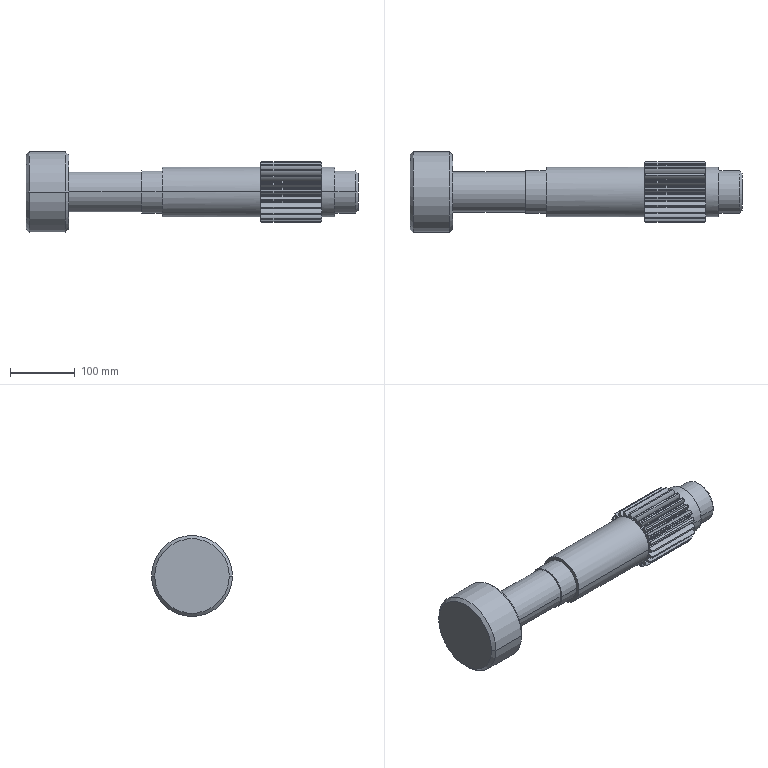Part | SolidWorks | features ICE 4, Fillet 2, Chamfer 1, Revolution 1, Scale 1 | 1 solid | 245 faces | box 511.875 x 125 x 125 mm | volume 2700404 mm3 | cylinder 140 | cone 53 | plane 52 | commonest cylinder face diameters 1.875 x57 29.625 x50 93.75 x23 65.625 x4 61.875 x2 76.875 x2